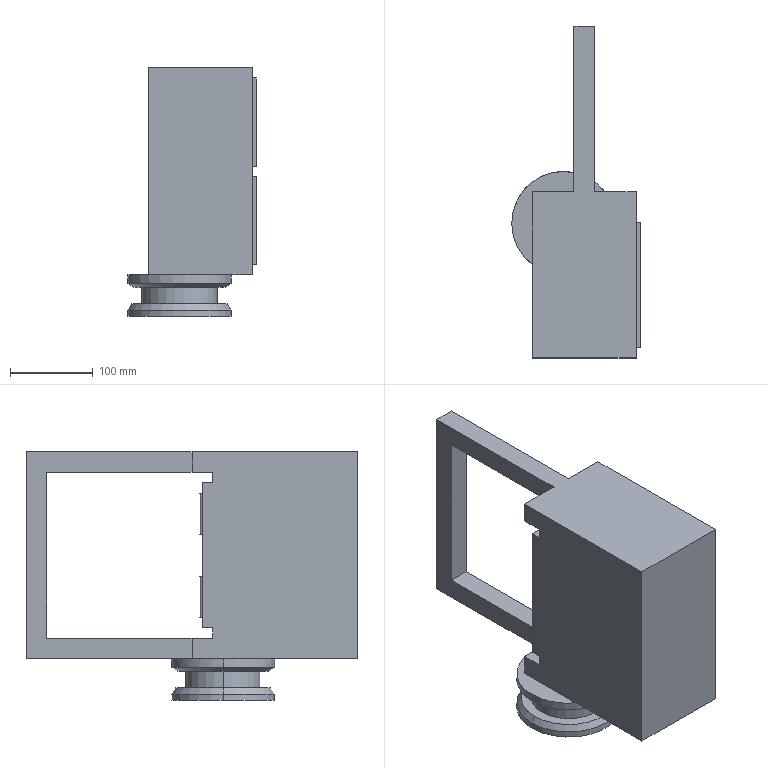Part | SolidWorks | features SplitBody 1 | 1 solid | 84 faces | box 155 x 400 x 300 mm | volume 6866912 mm3 | plane 66 | cylinder 14 | cone 4 | commonest cylinder face diameters 6.25 x8 125 x4 90.69 x2